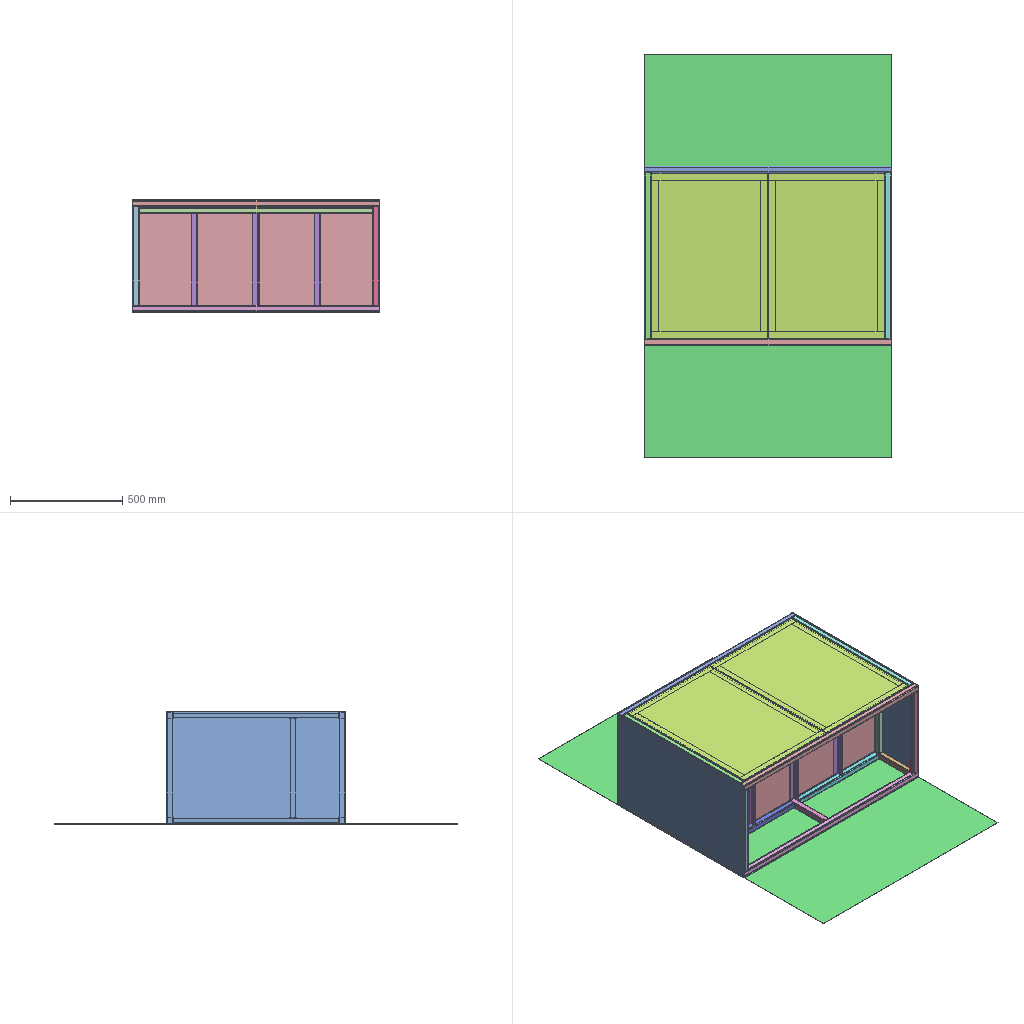Assembly | SolidWorks | 13 different items | 25 placed | box 1100 x 1797 x 500 mm
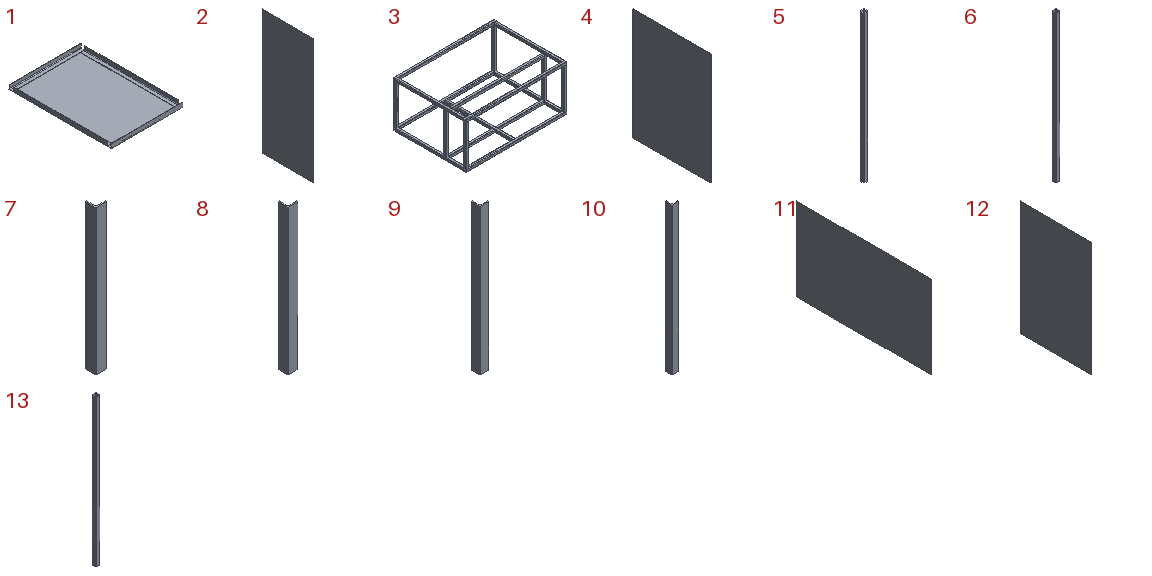Parts list (item | name | quantity | parent item | size | volume | features):
1 | (subassembly) | x2 | - | 515 x 735 x 31.2 mm | 870531 mm3 | features AEMSimFeature 1
2 | - | x1 | - | 1.2 x 437.6 x 1055 mm | 554002 mm3 | features FlatPattern 1, SMBaseFlange 1, SheetMetal 1
3 | - | x1 | - | 1098 x 797.6 x 498.8 mm | 3412994 mm3 | features 3DProfileFeature 1, WeldMemberFeat 1, WeldmentFeature 1
4 | - | x2 | in 1 | 1.2 x 515 x 735 mm | 454230 mm3 | features FlatPattern 1, SMBaseFlange 1, SheetMetal 1
5 | - | x1 | - | 30 x 30 x 1098 mm | 234556 mm3 | features Attribute 1, ExtruThin 1
6 | - | x1 | - | 30 x 30 x 1038 mm | 221734 mm3 | features Attribute 1, ExtruThin 1
7 | - | x3 | - | 30 x 30 x 407.6 mm | 71296 mm3 | features Extrusion 1
8 | - | x2 | - | 30 x 30 x 438.8 mm | 76753 mm3 | features Extrusion 1
9 | - | x4 | in 1 | 30 x 30 x 515 mm | 90082 mm3 | features Extrusion 1
10 | - | x4 | in 1 | 30 x 30 x 675 mm | 118069 mm3 | features Extrusion 1
11 | - | x1 | - | 1.2 x 1797 x 1100 mm | 2372141 mm3 | features FlatPattern 1, SMBaseFlange 1, SheetMetal 1, UnFold 1
12 | - | x2 | - | 1.2 x 498.8 x 797.6 mm | 477411 mm3 | features FlatPattern 1, SMBaseFlange 1, SheetMetal 1
13 | - | x1 | - | 30 x 30 x 1038 mm | 221734 mm3 | features Attribute 1, ExtruThin 1
Mates (type | each side: item.copy, entity, surface, feature):
In the top assembly
Coincident | 3.1 face plane Structural Member1 | 8.1 face plane Boss-Extrude1 | 2 times
DistanceDim | 8.1 face plane Boss-Extrude1 | 3.1 face plane Structural Member1
Coincident | 3.1 face plane Structural Member1 | 7.1 face plane Boss-Extrude1 | 2 times
DistanceDim | 7.1 face plane Boss-Extrude1 | 3.1 face plane Structural Member1
Coincident | 3.1 face plane Structural Member1 | 11.1 face plane Base-Flange1 | 2 times
DistanceDim | 3.1 face plane Structural Member1 | 11.1 face plane Base-Flange1
Coincident | 7.1 face plane Boss-Extrude1 | 2.1 face plane Base-Flange1
Coincident | 3.1 face plane Structural Member1 | 2.1 face plane Base-Flange1
Coincident | 11.1 plane | 2.1 plane
Coincident | 3.1 face plane Structural Member1 | 12.1 face plane Base-Flange1
Coincident | 11.1 face plane Base-Flange1 | 12.1 face plane Base-Flange1 | 2 times
Coincident | 3.1 face plane Structural Member1 | 12.2 face plane Base-Flange1
Coincident | 11.1 face plane Base-Flange1 | 12.2 face plane Base-Flange1 | 2 times
Coincident | 3.1 face plane Structural Member1 | 4.1 face plane Base-Flange1
DistanceDim | 9.1 face plane Boss-Extrude1 | 3.1 face plane Structural Member1
DistanceDim | 10.1 face plane Boss-Extrude1 | 3.1 face plane Structural Member1
In subassembly 1
Coincident | 4.2 face plane Base-Flange1 | 9.2 face plane Boss-Extrude1 | 3 times
Coincident | 4.2 face plane Base-Flange1 | 9.3 face plane Boss-Extrude1 | 3 times
Coincident | 4.2 face plane Base-Flange1 | 10.2 face plane Boss-Extrude1 | 2 times
Coincident | 9.2 face plane Boss-Extrude1 | 10.2 face plane Boss-Extrude1
Coincident | 4.2 face plane Base-Flange1 | 10.3 face plane Boss-Extrude1 | 2 times
Coincident | 9.2 face plane Boss-Extrude1 | 10.3 face plane Boss-Extrude1